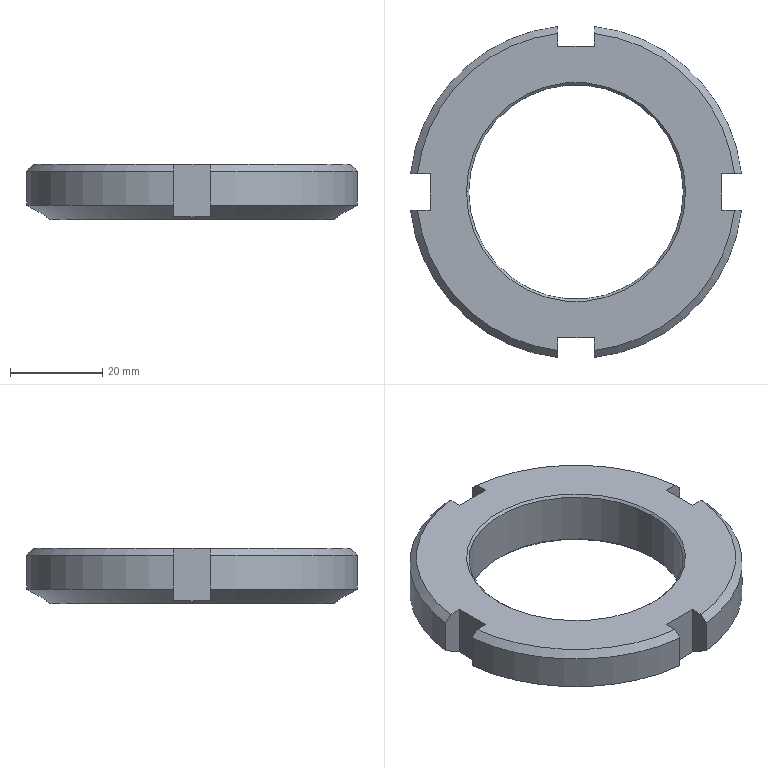Part | SolidWorks | features Chamfer 3, CirPattern 1, Cut 1, Extrusion 1 | 1 solid | 30 faces | box 71.554 x 71.554 x 12 mm | volume 25041 mm3 | plane 14 | cone 10 | cylinder 6 | commonest cylinder face diameters 72 x4 46.376 x2
STEP:
#1=CARTESIAN_POINT('',(-23.188,0.,11.5));
#2=VERTEX_POINT('',#1);
#3=CARTESIAN_POINT('',(23.188,0.,11.5));
#4=VERTEX_POINT('',#3);
#5=CARTESIAN_POINT('',(0.,0.,11.5));
#6=DIRECTION('',(0.,0.,1.));
#7=DIRECTION('',(1.,0.,0.));
#8=AXIS2_PLACEMENT_3D('',#5,#6,#7);
#9=CIRCLE('',#8,23.188);
#10=EDGE_CURVE('',#2,#4,#9,.T.);
#11=ORIENTED_EDGE('',*,*,#10,.F.);
#12=CARTESIAN_POINT('',(-23.688,0.,12.));
#13=VERTEX_POINT('',#12);
#14=CARTESIAN_POINT('',(-23.188,0.,11.5));
#15=DIRECTION('',(-0.7071,0.,0.7071));
#16=VECTOR('',#15,1000.);
#17=LINE('',#14,#16);
#18=EDGE_CURVE('',#2,#13,#17,.T.);
#19=ORIENTED_EDGE('',*,*,#18,.T.);
#20=CARTESIAN_POINT('',(23.688,0.,12.));
#21=VERTEX_POINT('',#20);
#22=CARTESIAN_POINT('',(0.,0.,12.));
#23=DIRECTION('',(0.,0.,-1.));
#24=DIRECTION('',(1.,0.,0.));
#25=AXIS2_PLACEMENT_3D('',#22,#23,#24);
#26=CIRCLE('',#25,23.688);
#27=EDGE_CURVE('',#21,#13,#26,.T.);
#28=ORIENTED_EDGE('',*,*,#27,.F.);
#29=CARTESIAN_POINT('',(23.188,0.,11.5));
#30=DIRECTION('',(0.7071,0.,0.7071));
#31=VECTOR('',#30,1000.);
#32=LINE('',#29,#31);
#33=EDGE_CURVE('',#4,#21,#32,.T.);
#34=ORIENTED_EDGE('',*,*,#33,.F.);
#35=EDGE_LOOP('',(#11,#19,#28,#34));
#36=FACE_OUTER_BOUND('',#35,.T.);
#37=CARTESIAN_POINT('',(0.,0.,11.5));
#38=DIRECTION('',(0.,0.,1.));
#39=DIRECTION('',(1.,0.,0.));
#40=AXIS2_PLACEMENT_3D('',#37,#38,#39);
#41=CONICAL_SURFACE('',#40,23.188,0.7854);
#42=ADVANCED_FACE('',(#36),#41,.F.);
#43=CARTESIAN_POINT('',(23.188,0.,0.5));
#44=VERTEX_POINT('',#43);
#45=CARTESIAN_POINT('',(-23.188,0.,0.5));
#46=VERTEX_POINT('',#45);
#47=CARTESIAN_POINT('',(0.,0.,0.5));
#48=DIRECTION('',(0.,0.,-1.));
#49=DIRECTION('',(1.,0.,0.));
#50=AXIS2_PLACEMENT_3D('',#47,#48,#49);
#51=CIRCLE('',#50,23.188);
#52=EDGE_CURVE('',#44,#46,#51,.T.);
#53=ORIENTED_EDGE('',*,*,#52,.F.);
#54=CARTESIAN_POINT('',(23.688,0.,0.));
#55=VERTEX_POINT('',#54);
#56=CARTESIAN_POINT('',(23.688,0.,0.));
#57=DIRECTION('',(0.7071,0.,-0.7071));
#58=VECTOR('',#57,1000.);
#59=LINE('',#56,#58);
#60=EDGE_CURVE('',#44,#55,#59,.T.);
#61=ORIENTED_EDGE('',*,*,#60,.T.);
#62=CARTESIAN_POINT('',(-23.688,0.,0.));
#63=VERTEX_POINT('',#62);
#64=CARTESIAN_POINT('',(0.,0.,0.));
#65=DIRECTION('',(0.,0.,1.));
#66=DIRECTION('',(1.,0.,0.));
#67=AXIS2_PLACEMENT_3D('',#64,#65,#66);
#68=CIRCLE('',#67,23.688);
#69=EDGE_CURVE('',#63,#55,#68,.T.);
#70=ORIENTED_EDGE('',*,*,#69,.F.);
#71=CARTESIAN_POINT('',(-23.688,0.,0.));
#72=DIRECTION('',(-0.7071,0.,-0.7071));
#73=VECTOR('',#72,1000.);
#74=LINE('',#71,#73);
#75=EDGE_CURVE('',#46,#63,#74,.T.);
#76=ORIENTED_EDGE('',*,*,#75,.F.);
#77=EDGE_LOOP('',(#53,#61,#70,#76));
#78=FACE_OUTER_BOUND('',#77,.T.);
#79=CARTESIAN_POINT('',(0.,0.,0.));
#80=DIRECTION('',(0.,0.,-1.));
#81=DIRECTION('',(-1.,0.,0.));
#82=AXIS2_PLACEMENT_3D('',#79,#80,#81);
#83=CONICAL_SURFACE('',#82,23.688,0.7854);
#84=ADVANCED_FACE('',(#78),#83,.F.);
#85=CARTESIAN_POINT('',(-30.5,0.,0.));
#86=VERTEX_POINT('',#85);
#87=CARTESIAN_POINT('',(30.5,0.,0.));
#88=VERTEX_POINT('',#87);
#89=CARTESIAN_POINT('',(0.,0.,0.));
#90=DIRECTION('',(0.,0.,-1.));
#91=DIRECTION('',(1.,0.,0.));
#92=AXIS2_PLACEMENT_3D('',#89,#90,#91);
#93=CIRCLE('',#92,30.5);
#94=EDGE_CURVE('',#86,#88,#93,.T.);
#95=ORIENTED_EDGE('',*,*,#94,.F.);
#96=CARTESIAN_POINT('',(-31.527,0.,0.593));
#97=VERTEX_POINT('',#96);
#98=CARTESIAN_POINT('',(-36.,0.,3.175));
#99=DIRECTION('',(-0.866,0.,0.5));
#100=VECTOR('',#99,1000.);
#101=LINE('',#98,#100);
#102=EDGE_CURVE('',#86,#97,#101,.T.);
#103=ORIENTED_EDGE('',*,*,#102,.T.);
#104=CARTESIAN_POINT('',(-31.527,4.,0.7389));
#105=VERTEX_POINT('',#104);
#106=CARTESIAN_POINT('',(-31.527,4.,0.7389));
#107=CARTESIAN_POINT('',(-31.527,2.671,0.6424));
#108=CARTESIAN_POINT('',(-31.527,1.338,0.593));
#109=CARTESIAN_POINT('',(-31.527,0.,0.593));
#110=B_SPLINE_CURVE_WITH_KNOTS('',3,(#106,#107,#108,#109),.UNSPECIFIED.,.F.,.F.,(4,4),(0.01045,0.01444),.UNSPECIFIED.);
#111=EDGE_CURVE('',#105,#97,#110,.T.);
#112=ORIENTED_EDGE('',*,*,#111,.F.);
#113=CARTESIAN_POINT('',(-35.777,4.,3.175));
#114=VERTEX_POINT('',#113);
#115=CARTESIAN_POINT('',(-35.777,4.,3.175));
#116=CARTESIAN_POINT('',(-34.361,4.,2.363));
#117=CARTESIAN_POINT('',(-32.944,4.,1.551));
#118=CARTESIAN_POINT('',(-31.527,4.,0.7389));
#119=B_SPLINE_CURVE_WITH_KNOTS('',3,(#115,#116,#117,#118),.UNSPECIFIED.,.F.,.F.,(4,4),(0.009232,0.01413),.UNSPECIFIED.);
#120=EDGE_CURVE('',#114,#105,#119,.T.);
#121=ORIENTED_EDGE('',*,*,#120,.F.);
#122=CARTESIAN_POINT('',(-4.,35.777,3.175));
#123=VERTEX_POINT('',#122);
#124=CARTESIAN_POINT('',(0.,0.,3.175));
#125=DIRECTION('',(0.,0.,1.));
#126=DIRECTION('',(1.,0.,0.));
#127=AXIS2_PLACEMENT_3D('',#124,#125,#126);
#128=CIRCLE('',#127,36.);
#129=EDGE_CURVE('',#123,#114,#128,.T.);
#130=ORIENTED_EDGE('',*,*,#129,.F.);
#131=CARTESIAN_POINT('',(-4.,31.527,0.7389));
#132=VERTEX_POINT('',#131);
#133=CARTESIAN_POINT('',(-4.,31.527,0.7389));
#134=CARTESIAN_POINT('',(-4.,32.944,1.551));
#135=CARTESIAN_POINT('',(-4.,34.361,2.363));
#136=CARTESIAN_POINT('',(-4.,35.777,3.175));
#137=B_SPLINE_CURVE_WITH_KNOTS('',3,(#133,#134,#135,#136),.UNSPECIFIED.,.F.,.F.,(4,4),(0.009599,0.0145),.UNSPECIFIED.);
#138=EDGE_CURVE('',#132,#123,#137,.T.);
#139=ORIENTED_EDGE('',*,*,#138,.F.);
#140=CARTESIAN_POINT('',(4.,31.527,0.7389));
#141=VERTEX_POINT('',#140);
#142=CARTESIAN_POINT('',(4.,31.527,0.7389));
#143=CARTESIAN_POINT('',(2.676,31.527,0.6427));
#144=CARTESIAN_POINT('',(1.347,31.527,0.5933));
#145=CARTESIAN_POINT('',(-0.6537,31.527,0.5928));
#146=CARTESIAN_POINT('',(-1.322,31.527,0.6049));
#147=CARTESIAN_POINT('',(-2.66,31.527,0.6536));
#148=CARTESIAN_POINT('',(-3.332,31.527,0.6903));
#149=CARTESIAN_POINT('',(-4.,31.527,0.7389));
#150=B_SPLINE_CURVE_WITH_KNOTS('',3,(#142,#143,#144,#145,#146,#147,#148,#149),.UNSPECIFIED.,.F.,.F.,(4,2,2,4),(0.01045,0.01443,0.01642,0.01841),.UNSPECIFIED.);
#151=EDGE_CURVE('',#141,#132,#150,.T.);
#152=ORIENTED_EDGE('',*,*,#151,.F.);
#153=CARTESIAN_POINT('',(4.,35.777,3.175));
#154=VERTEX_POINT('',#153);
#155=CARTESIAN_POINT('',(4.,35.777,3.175));
#156=CARTESIAN_POINT('',(4.,34.361,2.363));
#157=CARTESIAN_POINT('',(4.,32.944,1.551));
#158=CARTESIAN_POINT('',(4.,31.527,0.7389));
#159=B_SPLINE_CURVE_WITH_KNOTS('',3,(#155,#156,#157,#158),.UNSPECIFIED.,.F.,.F.,(4,4),(0.005677,0.01058),.UNSPECIFIED.);
#160=EDGE_CURVE('',#154,#141,#159,.T.);
#161=ORIENTED_EDGE('',*,*,#160,.F.);
#162=CARTESIAN_POINT('',(35.777,4.,3.175));
#163=VERTEX_POINT('',#162);
#164=CARTESIAN_POINT('',(0.,0.,3.175));
#165=DIRECTION('',(0.,0.,1.));
#166=DIRECTION('',(1.,0.,0.));
#167=AXIS2_PLACEMENT_3D('',#164,#165,#166);
#168=CIRCLE('',#167,36.);
#169=EDGE_CURVE('',#163,#154,#168,.T.);
#170=ORIENTED_EDGE('',*,*,#169,.F.);
#171=CARTESIAN_POINT('',(31.527,4.,0.7389));
#172=VERTEX_POINT('',#171);
#173=CARTESIAN_POINT('',(31.527,4.,0.7389));
#174=CARTESIAN_POINT('',(32.944,4.,1.551));
#175=CARTESIAN_POINT('',(34.361,4.,2.363));
#176=CARTESIAN_POINT('',(35.777,4.,3.175));
#177=B_SPLINE_CURVE_WITH_KNOTS('',3,(#173,#174,#175,#176),.UNSPECIFIED.,.F.,.F.,(4,4),(0.009599,0.0145),.UNSPECIFIED.);
#178=EDGE_CURVE('',#172,#163,#177,.T.);
#179=ORIENTED_EDGE('',*,*,#178,.F.);
#180=CARTESIAN_POINT('',(31.527,0.,0.593));
#181=VERTEX_POINT('',#180);
#182=CARTESIAN_POINT('',(31.527,0.,0.593));
#183=CARTESIAN_POINT('',(31.527,1.338,0.593));
#184=CARTESIAN_POINT('',(31.527,2.671,0.6424));
#185=CARTESIAN_POINT('',(31.527,4.,0.7389));
#186=B_SPLINE_CURVE_WITH_KNOTS('',3,(#182,#183,#184,#185),.UNSPECIFIED.,.F.,.F.,(4,4),(0.02046,0.02447),.UNSPECIFIED.);
#187=EDGE_CURVE('',#181,#172,#186,.T.);
#188=ORIENTED_EDGE('',*,*,#187,.F.);
#189=CARTESIAN_POINT('',(36.,0.,3.175));
#190=DIRECTION('',(0.866,0.,0.5));
#191=VECTOR('',#190,1000.);
#192=LINE('',#189,#191);
#193=EDGE_CURVE('',#88,#181,#192,.T.);
#194=ORIENTED_EDGE('',*,*,#193,.F.);
#195=EDGE_LOOP('',(#95,#103,#112,#121,#130,#139,#152,#161,#170,#179,#188,#194));
#196=FACE_OUTER_BOUND('',#195,.T.);
#197=CARTESIAN_POINT('',(0.,0.,3.175));
#198=DIRECTION('',(0.,0.,1.));
#199=DIRECTION('',(1.,0.,0.));
#200=AXIS2_PLACEMENT_3D('',#197,#198,#199);
#201=CONICAL_SURFACE('',#200,36.,1.047);
#202=ADVANCED_FACE('',(#196),#201,.T.);
#203=ORIENTED_EDGE('',*,*,#10,.T.);
#204=CARTESIAN_POINT('',(23.188,0.,12.));
#205=DIRECTION('',(0.,0.,-1.));
#206=VECTOR('',#205,1000.);
#207=LINE('',#204,#206);
#208=EDGE_CURVE('',#4,#44,#207,.T.);
#209=ORIENTED_EDGE('',*,*,#208,.T.);
#210=ORIENTED_EDGE('',*,*,#52,.T.);
#211=CARTESIAN_POINT('',(-23.188,0.,12.));
#212=DIRECTION('',(0.,0.,-1.));
#213=VECTOR('',#212,1000.);
#214=LINE('',#211,#213);
#215=EDGE_CURVE('',#2,#46,#214,.T.);
#216=ORIENTED_EDGE('',*,*,#215,.F.);
#217=EDGE_LOOP('',(#203,#209,#210,#216));
#218=FACE_OUTER_BOUND('',#217,.T.);
#219=CARTESIAN_POINT('',(0.,0.,12.));
#220=DIRECTION('',(0.,0.,-1.));
#221=DIRECTION('',(-1.,0.,0.));
#222=AXIS2_PLACEMENT_3D('',#219,#220,#221);
#223=CYLINDRICAL_SURFACE('',#222,23.188);
#224=ADVANCED_FACE('',(#218),#223,.F.);
#225=CARTESIAN_POINT('',(4.,35.777,10.5));
#226=VERTEX_POINT('',#225);
#227=CARTESIAN_POINT('',(35.777,4.,10.5));
#228=VERTEX_POINT('',#227);
#229=CARTESIAN_POINT('',(0.,0.,10.5));
#230=DIRECTION('',(0.,0.,-1.));
#231=DIRECTION('',(1.,0.,0.));
#232=AXIS2_PLACEMENT_3D('',#229,#230,#231);
#233=CIRCLE('',#232,36.);
#234=EDGE_CURVE('',#226,#228,#233,.T.);
#235=ORIENTED_EDGE('',*,*,#234,.T.);
#236=CARTESIAN_POINT('',(35.777,4.,0.));
#237=DIRECTION('',(0.,0.,1.));
#238=VECTOR('',#237,1000.);
#239=LINE('',#236,#238);
#240=EDGE_CURVE('',#163,#228,#239,.T.);
#241=ORIENTED_EDGE('',*,*,#240,.F.);
#242=ORIENTED_EDGE('',*,*,#169,.T.);
#243=CARTESIAN_POINT('',(4.,35.777,0.));
#244=DIRECTION('',(0.,0.,1.));
#245=VECTOR('',#244,1000.);
#246=LINE('',#243,#245);
#247=EDGE_CURVE('',#154,#226,#246,.T.);
#248=ORIENTED_EDGE('',*,*,#247,.T.);
#249=EDGE_LOOP('',(#235,#241,#242,#248));
#250=FACE_OUTER_BOUND('',#249,.T.);
#251=CARTESIAN_POINT('',(0.,0.,12.));
#252=DIRECTION('',(0.,0.,-1.));
#253=DIRECTION('',(-1.,0.,0.));
#254=AXIS2_PLACEMENT_3D('',#251,#252,#253);
#255=CYLINDRICAL_SURFACE('',#254,36.);
#256=ADVANCED_FACE('',(#250),#255,.T.);
#257=CARTESIAN_POINT('',(34.267,4.,12.));
#258=VERTEX_POINT('',#257);
#259=CARTESIAN_POINT('',(35.777,4.,10.5));
#260=CARTESIAN_POINT('',(35.385,4.,10.89));
#261=CARTESIAN_POINT('',(34.992,4.,11.28));
#262=CARTESIAN_POINT('',(34.6,4.,11.67));
#263=CARTESIAN_POINT('',(34.489,4.,11.78));
#264=CARTESIAN_POINT('',(34.378,4.,11.89));
#265=CARTESIAN_POINT('',(34.267,4.,12.));
#266=B_SPLINE_CURVE_WITH_KNOTS('',3,(#259,#260,#261,#262,#263,#264,#265),.UNSPECIFIED.,.F.,.F.,(4,3,4),(0.007216,0.008875,0.009344),.UNSPECIFIED.);
#267=EDGE_CURVE('',#228,#258,#266,.T.);
#268=ORIENTED_EDGE('',*,*,#267,.F.);
#269=ORIENTED_EDGE('',*,*,#234,.F.);
#270=CARTESIAN_POINT('',(4.,34.267,12.));
#271=VERTEX_POINT('',#270);
#272=CARTESIAN_POINT('',(4.,34.267,12.));
#273=CARTESIAN_POINT('',(4.,34.378,11.89));
#274=CARTESIAN_POINT('',(4.,34.489,11.78));
#275=CARTESIAN_POINT('',(4.,34.6,11.67));
#276=CARTESIAN_POINT('',(4.,34.992,11.28));
#277=CARTESIAN_POINT('',(4.,35.385,10.89));
#278=CARTESIAN_POINT('',(4.,35.777,10.5));
#279=B_SPLINE_CURVE_WITH_KNOTS('',3,(#272,#273,#274,#275,#276,#277,#278),.UNSPECIFIED.,.F.,.F.,(4,3,4),(0.008406,0.008875,0.01053),.UNSPECIFIED.);
#280=EDGE_CURVE('',#271,#226,#279,.T.);
#281=ORIENTED_EDGE('',*,*,#280,.F.);
#282=CARTESIAN_POINT('',(0.,0.,12.));
#283=DIRECTION('',(0.,0.,1.));
#284=DIRECTION('',(1.,0.,0.));
#285=AXIS2_PLACEMENT_3D('',#282,#283,#284);
#286=CIRCLE('',#285,34.5);
#287=EDGE_CURVE('',#258,#271,#286,.T.);
#288=ORIENTED_EDGE('',*,*,#287,.F.);
#289=EDGE_LOOP('',(#268,#269,#281,#288));
#290=FACE_OUTER_BOUND('',#289,.T.);
#291=CARTESIAN_POINT('',(0.,0.,12.));
#292=DIRECTION('',(0.,0.,-1.));
#293=DIRECTION('',(-1.,0.,0.));
#294=AXIS2_PLACEMENT_3D('',#291,#292,#293);
#295=CONICAL_SURFACE('',#294,34.5,0.7854);
#296=ADVANCED_FACE('',(#290),#295,.T.);
#297=CARTESIAN_POINT('',(-35.777,4.,10.5));
#298=VERTEX_POINT('',#297);
#299=CARTESIAN_POINT('',(-4.,35.777,10.5));
#300=VERTEX_POINT('',#299);
#301=CARTESIAN_POINT('',(0.,0.,10.5));
#302=DIRECTION('',(0.,0.,-1.));
#303=DIRECTION('',(1.,0.,0.));
#304=AXIS2_PLACEMENT_3D('',#301,#302,#303);
#305=CIRCLE('',#304,36.);
#306=EDGE_CURVE('',#298,#300,#305,.T.);
#307=ORIENTED_EDGE('',*,*,#306,.T.);
#308=CARTESIAN_POINT('',(-4.,35.777,0.));
#309=DIRECTION('',(0.,0.,1.));
#310=VECTOR('',#309,1000.);
#311=LINE('',#308,#310);
#312=EDGE_CURVE('',#123,#300,#311,.T.);
#313=ORIENTED_EDGE('',*,*,#312,.F.);
#314=ORIENTED_EDGE('',*,*,#129,.T.);
#315=CARTESIAN_POINT('',(-35.777,4.,0.));
#316=DIRECTION('',(0.,0.,1.));
#317=VECTOR('',#316,1000.);
#318=LINE('',#315,#317);
#319=EDGE_CURVE('',#114,#298,#318,.T.);
#320=ORIENTED_EDGE('',*,*,#319,.T.);
#321=EDGE_LOOP('',(#307,#313,#314,#320));
#322=FACE_OUTER_BOUND('',#321,.T.);
#323=CARTESIAN_POINT('',(0.,0.,12.));
#324=DIRECTION('',(0.,0.,-1.));
#325=DIRECTION('',(-1.,0.,0.));
#326=AXIS2_PLACEMENT_3D('',#323,#324,#325);
#327=CYLINDRICAL_SURFACE('',#326,36.);
#328=ADVANCED_FACE('',(#322),#327,.T.);
#329=CARTESIAN_POINT('',(-4.,34.267,12.));
#330=VERTEX_POINT('',#329);
#331=CARTESIAN_POINT('',(-4.,35.777,10.5));
#332=CARTESIAN_POINT('',(-4.,35.385,10.89));
#333=CARTESIAN_POINT('',(-4.,34.992,11.28));
#334=CARTESIAN_POINT('',(-4.,34.6,11.67));
#335=CARTESIAN_POINT('',(-4.,34.489,11.78));
#336=CARTESIAN_POINT('',(-4.,34.378,11.89));
#337=CARTESIAN_POINT('',(-4.,34.267,12.));
#338=B_SPLINE_CURVE_WITH_KNOTS('',3,(#331,#332,#333,#334,#335,#336,#337),.UNSPECIFIED.,.F.,.F.,(4,3,4),(0.007216,0.008875,0.009344),.UNSPECIFIED.);
#339=EDGE_CURVE('',#300,#330,#338,.T.);
#340=ORIENTED_EDGE('',*,*,#339,.F.);
#341=ORIENTED_EDGE('',*,*,#306,.F.);
#342=CARTESIAN_POINT('',(-34.267,4.,12.));
#343=VERTEX_POINT('',#342);
#344=CARTESIAN_POINT('',(-34.267,4.,12.));
#345=CARTESIAN_POINT('',(-34.557,4.,11.713));
#346=CARTESIAN_POINT('',(-34.846,4.,11.426));
#347=CARTESIAN_POINT('',(-35.135,4.,11.138));
#348=CARTESIAN_POINT('',(-35.349,4.,10.926));
#349=CARTESIAN_POINT('',(-35.563,4.,10.713));
#350=CARTESIAN_POINT('',(-35.777,4.,10.5));
#351=B_SPLINE_CURVE_WITH_KNOTS('',3,(#344,#345,#346,#347,#348,#349,#350),.UNSPECIFIED.,.F.,.F.,(4,3,4),(0.007653,0.008875,0.009781),.UNSPECIFIED.);
#352=EDGE_CURVE('',#343,#298,#351,.T.);
#353=ORIENTED_EDGE('',*,*,#352,.F.);
#354=CARTESIAN_POINT('',(0.,0.,12.));
#355=DIRECTION('',(0.,0.,1.));
#356=DIRECTION('',(1.,0.,0.));
#357=AXIS2_PLACEMENT_3D('',#354,#355,#356);
#358=CIRCLE('',#357,34.5);
#359=EDGE_CURVE('',#330,#343,#358,.T.);
#360=ORIENTED_EDGE('',*,*,#359,.F.);
#361=EDGE_LOOP('',(#340,#341,#353,#360));
#362=FACE_OUTER_BOUND('',#361,.T.);
#363=CARTESIAN_POINT('',(0.,0.,12.));
#364=DIRECTION('',(0.,0.,-1.));
#365=DIRECTION('',(-1.,0.,0.));
#366=AXIS2_PLACEMENT_3D('',#363,#364,#365);
#367=CONICAL_SURFACE('',#366,34.5,0.7854);
#368=ADVANCED_FACE('',(#362),#367,.T.);
#369=CARTESIAN_POINT('',(-4.,-35.777,10.5));
#370=VERTEX_POINT('',#369);
#371=CARTESIAN_POINT('',(-35.777,-4.,10.5));
#372=VERTEX_POINT('',#371);
#373=CARTESIAN_POINT('',(0.,0.,10.5));
#374=DIRECTION('',(0.,0.,-1.));
#375=DIRECTION('',(1.,0.,0.));
#376=AXIS2_PLACEMENT_3D('',#373,#374,#375);
#377=CIRCLE('',#376,36.);
#378=EDGE_CURVE('',#370,#372,#377,.T.);
#379=ORIENTED_EDGE('',*,*,#378,.T.);
#380=CARTESIAN_POINT('',(-35.777,-4.,3.175));
#381=VERTEX_POINT('',#380);
#382=CARTESIAN_POINT('',(-35.777,-4.,0.));
#383=DIRECTION('',(0.,0.,1.));
#384=VECTOR('',#383,1000.);
#385=LINE('',#382,#384);
#386=EDGE_CURVE('',#381,#372,#385,.T.);
#387=ORIENTED_EDGE('',*,*,#386,.F.);
#388=CARTESIAN_POINT('',(-4.,-35.777,3.175));
#389=VERTEX_POINT('',#388);
#390=CARTESIAN_POINT('',(0.,0.,3.175));
#391=DIRECTION('',(0.,0.,1.));
#392=DIRECTION('',(1.,0.,0.));
#393=AXIS2_PLACEMENT_3D('',#390,#391,#392);
#394=CIRCLE('',#393,36.);
#395=EDGE_CURVE('',#381,#389,#394,.T.);
#396=ORIENTED_EDGE('',*,*,#395,.T.);
#397=CARTESIAN_POINT('',(-4.,-35.777,0.));
#398=DIRECTION('',(0.,0.,1.));
#399=VECTOR('',#398,1000.);
#400=LINE('',#397,#399);
#401=EDGE_CURVE('',#389,#370,#400,.T.);
#402=ORIENTED_EDGE('',*,*,#401,.T.);
#403=EDGE_LOOP('',(#379,#387,#396,#402));
#404=FACE_OUTER_BOUND('',#403,.T.);
#405=CARTESIAN_POINT('',(0.,0.,12.));
#406=DIRECTION('',(0.,0.,-1.));
#407=DIRECTION('',(-1.,0.,0.));
#408=AXIS2_PLACEMENT_3D('',#405,#406,#407);
#409=CYLINDRICAL_SURFACE('',#408,36.);
#410=ADVANCED_FACE('',(#404),#409,.T.);
#411=CARTESIAN_POINT('',(-34.267,-4.,12.));
#412=VERTEX_POINT('',#411);
#413=CARTESIAN_POINT('',(-35.777,-4.,10.5));
#414=CARTESIAN_POINT('',(-35.563,-4.,10.713));
#415=CARTESIAN_POINT('',(-35.349,-4.,10.926));
#416=CARTESIAN_POINT('',(-35.135,-4.,11.138));
#417=CARTESIAN_POINT('',(-34.846,-4.,11.426));
#418=CARTESIAN_POINT('',(-34.557,-4.,11.713));
#419=CARTESIAN_POINT('',(-34.267,-4.,12.));
#420=B_SPLINE_CURVE_WITH_KNOTS('',3,(#413,#414,#415,#416,#417,#418,#419),.UNSPECIFIED.,.F.,.F.,(4,3,4),(0.00797,0.008875,0.0101),.UNSPECIFIED.);
#421=EDGE_CURVE('',#372,#412,#420,.T.);
#422=ORIENTED_EDGE('',*,*,#421,.F.);
#423=ORIENTED_EDGE('',*,*,#378,.F.);
#424=CARTESIAN_POINT('',(-4.,-34.267,12.));
#425=VERTEX_POINT('',#424);
#426=CARTESIAN_POINT('',(-4.,-34.267,12.));
#427=CARTESIAN_POINT('',(-4.,-34.557,11.713));
#428=CARTESIAN_POINT('',(-4.,-34.846,11.426));
#429=CARTESIAN_POINT('',(-4.,-35.135,11.138));
#430=CARTESIAN_POINT('',(-4.,-35.349,10.926));
#431=CARTESIAN_POINT('',(-4.,-35.563,10.713));
#432=CARTESIAN_POINT('',(-4.,-35.777,10.5));
#433=B_SPLINE_CURVE_WITH_KNOTS('',3,(#426,#427,#428,#429,#430,#431,#432),.UNSPECIFIED.,.F.,.F.,(4,3,4),(0.007653,0.008875,0.009781),.UNSPECIFIED.);
#434=EDGE_CURVE('',#425,#370,#433,.T.);
#435=ORIENTED_EDGE('',*,*,#434,.F.);
#436=CARTESIAN_POINT('',(0.,0.,12.));
#437=DIRECTION('',(0.,0.,1.));
#438=DIRECTION('',(1.,0.,0.));
#439=AXIS2_PLACEMENT_3D('',#436,#437,#438);
#440=CIRCLE('',#439,34.5);
#441=EDGE_CURVE('',#412,#425,#440,.T.);
#442=ORIENTED_EDGE('',*,*,#441,.F.);
#443=EDGE_LOOP('',(#422,#423,#435,#442));
#444=FACE_OUTER_BOUND('',#443,.T.);
#445=CARTESIAN_POINT('',(0.,0.,12.));
#446=DIRECTION('',(0.,0.,-1.));
#447=DIRECTION('',(-1.,0.,0.));
#448=AXIS2_PLACEMENT_3D('',#445,#446,#447);
#449=CONICAL_SURFACE('',#448,34.5,0.7854);
#450=ADVANCED_FACE('',(#444),#449,.T.);
#451=ORIENTED_EDGE('',*,*,#27,.T.);
#452=CARTESIAN_POINT('',(0.,0.,12.));
#453=DIRECTION('',(0.,0.,-1.));
#454=DIRECTION('',(1.,0.,0.));
#455=AXIS2_PLACEMENT_3D('',#452,#453,#454);
#456=CIRCLE('',#455,23.688);
#457=EDGE_CURVE('',#13,#21,#456,.T.);
#458=ORIENTED_EDGE('',*,*,#457,.T.);
#459=EDGE_LOOP('',(#451,#458));
#460=FACE_BOUND('',#459,.T.);
#461=CARTESIAN_POINT('',(31.527,4.,12.));
#462=VERTEX_POINT('',#461);
#463=CARTESIAN_POINT('',(31.527,4.,12.));
#464=DIRECTION('',(-1.,0.,0.));
#465=VECTOR('',#464,1000.);
#466=LINE('',#463,#465);
#467=EDGE_CURVE('',#258,#462,#466,.T.);
#468=ORIENTED_EDGE('',*,*,#467,.F.);
#469=ORIENTED_EDGE('',*,*,#287,.T.);
#470=CARTESIAN_POINT('',(4.,31.527,12.));
#471=VERTEX_POINT('',#470);
#472=CARTESIAN_POINT('',(4.,31.527,12.));
#473=DIRECTION('',(0.,1.,0.));
#474=VECTOR('',#473,1000.);
#475=LINE('',#472,#474);
#476=EDGE_CURVE('',#471,#271,#475,.T.);
#477=ORIENTED_EDGE('',*,*,#476,.F.);
#478=CARTESIAN_POINT('',(-4.,31.527,12.));
#479=VERTEX_POINT('',#478);
#480=CARTESIAN_POINT('',(4.,31.527,12.));
#481=DIRECTION('',(1.,0.,0.));
#482=VECTOR('',#481,1000.);
#483=LINE('',#480,#482);
#484=EDGE_CURVE('',#479,#471,#483,.T.);
#485=ORIENTED_EDGE('',*,*,#484,.F.);
#486=CARTESIAN_POINT('',(-4.,31.527,12.));
#487=DIRECTION('',(0.,-1.,0.));
#488=VECTOR('',#487,1000.);
#489=LINE('',#486,#488);
#490=EDGE_CURVE('',#330,#479,#489,.T.);
#491=ORIENTED_EDGE('',*,*,#490,.F.);
#492=ORIENTED_EDGE('',*,*,#359,.T.);
#493=CARTESIAN_POINT('',(-31.527,4.,12.));
#494=VERTEX_POINT('',#493);
#495=CARTESIAN_POINT('',(-31.527,4.,12.));
#496=DIRECTION('',(-1.,0.,0.));
#497=VECTOR('',#496,1000.);
#498=LINE('',#495,#497);
#499=EDGE_CURVE('',#494,#343,#498,.T.);
#500=ORIENTED_EDGE('',*,*,#499,.F.);
#501=CARTESIAN_POINT('',(-31.527,-4.,12.));
#502=VERTEX_POINT('',#501);
#503=CARTESIAN_POINT('',(-31.527,4.,12.));
#504=DIRECTION('',(0.,1.,0.));
#505=VECTOR('',#504,1000.);
#506=LINE('',#503,#505);
#507=EDGE_CURVE('',#502,#494,#506,.T.);
#508=ORIENTED_EDGE('',*,*,#507,.F.);
#509=CARTESIAN_POINT('',(-31.527,-4.,12.));
#510=DIRECTION('',(1.,0.,0.));
#511=VECTOR('',#510,1000.);
#512=LINE('',#509,#511);
#513=EDGE_CURVE('',#412,#502,#512,.T.);
#514=ORIENTED_EDGE('',*,*,#513,.F.);
#515=ORIENTED_EDGE('',*,*,#441,.T.);
#516=CARTESIAN_POINT('',(-4.,-31.527,12.));
#517=VERTEX_POINT('',#516);
#518=CARTESIAN_POINT('',(-4.,-31.527,12.));
#519=DIRECTION('',(0.,-1.,0.));
#520=VECTOR('',#519,1000.);
#521=LINE('',#518,#520);
#522=EDGE_CURVE('',#517,#425,#521,.T.);
#523=ORIENTED_EDGE('',*,*,#522,.F.);
#524=CARTESIAN_POINT('',(4.,-31.527,12.));
#525=VERTEX_POINT('',#524);
#526=CARTESIAN_POINT('',(-4.,-31.527,12.));
#527=DIRECTION('',(-1.,0.,0.));
#528=VECTOR('',#527,1000.);
#529=LINE('',#526,#528);
#530=EDGE_CURVE('',#525,#517,#529,.T.);
#531=ORIENTED_EDGE('',*,*,#530,.F.);
#532=CARTESIAN_POINT('',(4.,-34.267,12.));
#533=VERTEX_POINT('',#532);
#534=CARTESIAN_POINT('',(4.,-31.527,12.));
#535=DIRECTION('',(0.,1.,0.));
#536=VECTOR('',#535,1000.);
#537=LINE('',#534,#536);
#538=EDGE_CURVE('',#533,#525,#537,.T.);
#539=ORIENTED_EDGE('',*,*,#538,.F.);
#540=CARTESIAN_POINT('',(34.267,-4.,12.));
#541=VERTEX_POINT('',#540);
#542=CARTESIAN_POINT('',(0.,0.,12.));
#543=DIRECTION('',(0.,0.,1.));
#544=DIRECTION('',(1.,0.,0.));
#545=AXIS2_PLACEMENT_3D('',#542,#543,#544);
#546=CIRCLE('',#545,34.5);
#547=EDGE_CURVE('',#533,#541,#546,.T.);
#548=ORIENTED_EDGE('',*,*,#547,.T.);
#549=CARTESIAN_POINT('',(31.527,-4.,12.));
#550=VERTEX_POINT('',#549);
#551=CARTESIAN_POINT('',(31.527,-4.,12.));
#552=DIRECTION('',(1.,0.,0.));
#553=VECTOR('',#552,1000.);
#554=LINE('',#551,#553);
#555=EDGE_CURVE('',#550,#541,#554,.T.);
#556=ORIENTED_EDGE('',*,*,#555,.F.);
#557=CARTESIAN_POINT('',(31.527,-4.,12.));
#558=DIRECTION('',(0.,-1.,0.));
#559=VECTOR('',#558,1000.);
#560=LINE('',#557,#559);
#561=EDGE_CURVE('',#462,#550,#560,.T.);
#562=ORIENTED_EDGE('',*,*,#561,.F.);
#563=EDGE_LOOP('',(#468,#469,#477,#485,#491,#492,#500,#508,#514,#515,#523,#531,#539,#548,#556,#562));
#564=FACE_OUTER_BOUND('',#563,.T.);
#565=CARTESIAN_POINT('',(0.,0.,12.));
#566=DIRECTION('',(0.,0.,1.));
#567=DIRECTION('',(1.,0.,0.));
#568=AXIS2_PLACEMENT_3D('',#565,#566,#567);
#569=PLANE('',#568);
#570=ADVANCED_FACE('',(#460,#564),#569,.T.);
#571=ORIENTED_EDGE('',*,*,#69,.T.);
#572=CARTESIAN_POINT('',(0.,0.,0.));
#573=DIRECTION('',(0.,0.,1.));
#574=DIRECTION('',(1.,0.,0.));
#575=AXIS2_PLACEMENT_3D('',#572,#573,#574);
#576=CIRCLE('',#575,23.688);
#577=EDGE_CURVE('',#55,#63,#576,.T.);
#578=ORIENTED_EDGE('',*,*,#577,.T.);
#579=EDGE_LOOP('',(#571,#578));
#580=FACE_BOUND('',#579,.T.);
#581=CARTESIAN_POINT('',(0.,0.,0.));
#582=DIRECTION('',(0.,0.,-1.));
#583=DIRECTION('',(1.,0.,0.));
#584=AXIS2_PLACEMENT_3D('',#581,#582,#583);
#585=CIRCLE('',#584,30.5);
#586=EDGE_CURVE('',#88,#86,#585,.T.);
#587=ORIENTED_EDGE('',*,*,#586,.T.);
#588=ORIENTED_EDGE('',*,*,#94,.T.);
#589=EDGE_LOOP('',(#587,#588));
#590=FACE_OUTER_BOUND('',#589,.T.);
#591=CARTESIAN_POINT('',(0.,0.,0.));
#592=DIRECTION('',(0.,0.,1.));
#593=DIRECTION('',(1.,0.,0.));
#594=AXIS2_PLACEMENT_3D('',#591,#592,#593);
#595=PLANE('',#594);
#596=ADVANCED_FACE('',(#580,#590),#595,.F.);
#597=CARTESIAN_POINT('',(4.,-35.777,3.175));
#598=VERTEX_POINT('',#597);
#599=CARTESIAN_POINT('',(35.777,-4.,3.175));
#600=VERTEX_POINT('',#599);
#601=CARTESIAN_POINT('',(0.,0.,3.175));
#602=DIRECTION('',(0.,0.,1.));
#603=DIRECTION('',(1.,0.,0.));
#604=AXIS2_PLACEMENT_3D('',#601,#602,#603);
#605=CIRCLE('',#604,36.);
#606=EDGE_CURVE('',#598,#600,#605,.T.);
#607=ORIENTED_EDGE('',*,*,#606,.T.);
#608=CARTESIAN_POINT('',(35.777,-4.,10.5));
#609=VERTEX_POINT('',#608);
#610=CARTESIAN_POINT('',(35.777,-4.,0.));
#611=DIRECTION('',(0.,0.,1.));
#612=VECTOR('',#611,1000.);
#613=LINE('',#610,#612);
#614=EDGE_CURVE('',#600,#609,#613,.T.);
#615=ORIENTED_EDGE('',*,*,#614,.T.);
#616=CARTESIAN_POINT('',(4.,-35.777,10.5));
#617=VERTEX_POINT('',#616);
#618=CARTESIAN_POINT('',(0.,0.,10.5));
#619=DIRECTION('',(0.,0.,-1.));
#620=DIRECTION('',(1.,0.,0.));
#621=AXIS2_PLACEMENT_3D('',#618,#619,#620);
#622=CIRCLE('',#621,36.);
#623=EDGE_CURVE('',#609,#617,#622,.T.);
#624=ORIENTED_EDGE('',*,*,#623,.T.);
#625=CARTESIAN_POINT('',(4.,-35.777,0.));
#626=DIRECTION('',(0.,0.,1.));
#627=VECTOR('',#626,1000.);
#628=LINE('',#625,#627);
#629=EDGE_CURVE('',#598,#617,#628,.T.);
#630=ORIENTED_EDGE('',*,*,#629,.F.);
#631=EDGE_LOOP('',(#607,#615,#624,#630));
#632=FACE_OUTER_BOUND('',#631,.T.);
#633=CARTESIAN_POINT('',(0.,0.,12.));
#634=DIRECTION('',(0.,0.,-1.));
#635=DIRECTION('',(-1.,0.,0.));
#636=AXIS2_PLACEMENT_3D('',#633,#634,#635);
#637=CYLINDRICAL_SURFACE('',#636,36.);
#638=ADVANCED_FACE('',(#632),#637,.T.);
#639=ORIENTED_EDGE('',*,*,#208,.F.);
#640=CARTESIAN_POINT('',(0.,0.,11.5));
#641=DIRECTION('',(0.,0.,1.));
#642=DIRECTION('',(1.,0.,0.));
#643=AXIS2_PLACEMENT_3D('',#640,#641,#642);
#644=CIRCLE('',#643,23.188);
#645=EDGE_CURVE('',#4,#2,#644,.T.);
#646=ORIENTED_EDGE('',*,*,#645,.T.);
#647=ORIENTED_EDGE('',*,*,#215,.T.);
#648=CARTESIAN_POINT('',(0.,0.,0.5));
#649=DIRECTION('',(0.,0.,-1.));
#650=DIRECTION('',(1.,0.,0.));
#651=AXIS2_PLACEMENT_3D('',#648,#649,#650);
#652=CIRCLE('',#651,23.188);
#653=EDGE_CURVE('',#46,#44,#652,.T.);
#654=ORIENTED_EDGE('',*,*,#653,.T.);
#655=EDGE_LOOP('',(#639,#646,#647,#654));
#656=FACE_OUTER_BOUND('',#655,.T.);
#657=CARTESIAN_POINT('',(0.,0.,12.));
#658=DIRECTION('',(0.,0.,-1.));
#659=DIRECTION('',(-1.,0.,0.));
#660=AXIS2_PLACEMENT_3D('',#657,#658,#659);
#661=CYLINDRICAL_SURFACE('',#660,23.188);
#662=ADVANCED_FACE('',(#656),#661,.F.);
#663=CARTESIAN_POINT('',(34.267,-4.,12.));
#664=CARTESIAN_POINT('',(34.378,-4.,11.89));
#665=CARTESIAN_POINT('',(34.489,-4.,11.78));
#666=CARTESIAN_POINT('',(34.6,-4.,11.67));
#667=CARTESIAN_POINT('',(34.992,-4.,11.28));
#668=CARTESIAN_POINT('',(35.385,-4.,10.89));
#669=CARTESIAN_POINT('',(35.777,-4.,10.5));
#670=B_SPLINE_CURVE_WITH_KNOTS('',3,(#663,#664,#665,#666,#667,#668,#669),.UNSPECIFIED.,.F.,.F.,(4,3,4),(0.008406,0.008875,0.01053),.UNSPECIFIED.);
#671=EDGE_CURVE('',#541,#609,#670,.T.);
#672=ORIENTED_EDGE('',*,*,#671,.F.);
#673=ORIENTED_EDGE('',*,*,#547,.F.);
#674=CARTESIAN_POINT('',(4.,-35.777,10.5));
#675=CARTESIAN_POINT('',(4.,-35.563,10.713));
#676=CARTESIAN_POINT('',(4.,-35.349,10.926));
#677=CARTESIAN_POINT('',(4.,-35.135,11.138));
#678=CARTESIAN_POINT('',(4.,-34.846,11.426));
#679=CARTESIAN_POINT('',(4.,-34.557,11.713));
#680=CARTESIAN_POINT('',(4.,-34.267,12.));
#681=B_SPLINE_CURVE_WITH_KNOTS('',3,(#674,#675,#676,#677,#678,#679,#680),.UNSPECIFIED.,.F.,.F.,(4,3,4),(0.00797,0.008875,0.0101),.UNSPECIFIED.);
#682=EDGE_CURVE('',#617,#533,#681,.T.);
#683=ORIENTED_EDGE('',*,*,#682,.F.);
#684=ORIENTED_EDGE('',*,*,#623,.F.);
#685=EDGE_LOOP('',(#672,#673,#683,#684));
#686=FACE_OUTER_BOUND('',#685,.T.);
#687=CARTESIAN_POINT('',(0.,0.,12.));
#688=DIRECTION('',(0.,0.,-1.));
#689=DIRECTION('',(-1.,0.,0.));
#690=AXIS2_PLACEMENT_3D('',#687,#688,#689);
#691=CONICAL_SURFACE('',#690,34.5,0.7854);
#692=ADVANCED_FACE('',(#686),#691,.T.);
#693=ORIENTED_EDGE('',*,*,#102,.F.);
#694=ORIENTED_EDGE('',*,*,#586,.F.);
#695=ORIENTED_EDGE('',*,*,#193,.T.);
#696=CARTESIAN_POINT('',(31.527,-4.,0.7389));
#697=VERTEX_POINT('',#696);
#698=CARTESIAN_POINT('',(31.527,-4.,0.7389));
#699=CARTESIAN_POINT('',(31.527,-3.334,0.6905));
#700=CARTESIAN_POINT('',(31.527,-2.665,0.6538));
#701=CARTESIAN_POINT('',(31.527,-1.331,0.6051));
#702=CARTESIAN_POINT('',(31.527,-0.6647,0.593));
#703=CARTESIAN_POINT('',(31.527,0.,0.593));
#704=B_SPLINE_CURVE_WITH_KNOTS('',3,(#698,#699,#700,#701,#702,#703),.UNSPECIFIED.,.F.,.F.,(4,2,4),(0.01648,0.01847,0.02046),.UNSPECIFIED.);
#705=EDGE_CURVE('',#697,#181,#704,.T.);
#706=ORIENTED_EDGE('',*,*,#705,.F.);
#707=CARTESIAN_POINT('',(35.777,-4.,3.175));
#708=CARTESIAN_POINT('',(34.361,-4.,2.363));
#709=CARTESIAN_POINT('',(32.944,-4.,1.551));
#710=CARTESIAN_POINT('',(31.527,-4.,0.7389));
#711=B_SPLINE_CURVE_WITH_KNOTS('',3,(#707,#708,#709,#710),.UNSPECIFIED.,.F.,.F.,(4,4),(0.005677,0.01058),.UNSPECIFIED.);
#712=EDGE_CURVE('',#600,#697,#711,.T.);
#713=ORIENTED_EDGE('',*,*,#712,.F.);
#714=ORIENTED_EDGE('',*,*,#606,.F.);
#715=CARTESIAN_POINT('',(4.,-31.527,0.7389));
#716=VERTEX_POINT('',#715);
#717=CARTESIAN_POINT('',(4.,-31.527,0.7389));
#718=CARTESIAN_POINT('',(4.,-32.944,1.551));
#719=CARTESIAN_POINT('',(4.,-34.361,2.363));
#720=CARTESIAN_POINT('',(4.,-35.777,3.175));
#721=B_SPLINE_CURVE_WITH_KNOTS('',3,(#717,#718,#719,#720),.UNSPECIFIED.,.F.,.F.,(4,4),(0.006045,0.01094),.UNSPECIFIED.);
#722=EDGE_CURVE('',#716,#598,#721,.T.);
#723=ORIENTED_EDGE('',*,*,#722,.F.);
#724=CARTESIAN_POINT('',(-4.,-31.527,0.7389));
#725=VERTEX_POINT('',#724);
#726=CARTESIAN_POINT('',(-4.,-31.527,0.7389));
#727=CARTESIAN_POINT('',(-3.332,-31.527,0.6903));
#728=CARTESIAN_POINT('',(-2.66,-31.527,0.6536));
#729=CARTESIAN_POINT('',(-1.322,-31.527,0.6049));
#730=CARTESIAN_POINT('',(-0.6537,-31.527,0.5928));
#731=CARTESIAN_POINT('',(1.347,-31.527,0.5933));
#732=CARTESIAN_POINT('',(2.676,-31.527,0.6427));
#733=CARTESIAN_POINT('',(4.,-31.527,0.7389));
#734=B_SPLINE_CURVE_WITH_KNOTS('',3,(#726,#727,#728,#729,#730,#731,#732,#733),.UNSPECIFIED.,.F.,.F.,(4,2,2,4),(0.01648,0.01848,0.02047,0.02447),.UNSPECIFIED.);
#735=EDGE_CURVE('',#725,#716,#734,.T.);
#736=ORIENTED_EDGE('',*,*,#735,.F.);
#737=CARTESIAN_POINT('',(-4.,-35.777,3.175));
#738=CARTESIAN_POINT('',(-4.,-34.361,2.363));
#739=CARTESIAN_POINT('',(-4.,-32.944,1.551));
#740=CARTESIAN_POINT('',(-4.,-31.527,0.7389));
#741=B_SPLINE_CURVE_WITH_KNOTS('',3,(#737,#738,#739,#740),.UNSPECIFIED.,.F.,.F.,(4,4),(0.009232,0.01413),.UNSPECIFIED.);
#742=EDGE_CURVE('',#389,#725,#741,.T.);
#743=ORIENTED_EDGE('',*,*,#742,.F.);
#744=ORIENTED_EDGE('',*,*,#395,.F.);
#745=CARTESIAN_POINT('',(-31.527,-4.,0.7389));
#746=VERTEX_POINT('',#745);
#747=CARTESIAN_POINT('',(-31.527,-4.,0.7389));
#748=CARTESIAN_POINT('',(-32.944,-4.,1.551));
#749=CARTESIAN_POINT('',(-34.361,-4.,2.363));
#750=CARTESIAN_POINT('',(-35.777,-4.,3.175));
#751=B_SPLINE_CURVE_WITH_KNOTS('',3,(#747,#748,#749,#750),.UNSPECIFIED.,.F.,.F.,(4,4),(0.006045,0.01094),.UNSPECIFIED.);
#752=EDGE_CURVE('',#746,#381,#751,.T.);
#753=ORIENTED_EDGE('',*,*,#752,.F.);
#754=CARTESIAN_POINT('',(-31.527,0.,0.593));
#755=CARTESIAN_POINT('',(-31.527,-0.6647,0.593));
#756=CARTESIAN_POINT('',(-31.527,-1.331,0.6051));
#757=CARTESIAN_POINT('',(-31.527,-2.665,0.6538));
#758=CARTESIAN_POINT('',(-31.527,-3.334,0.6905));
#759=CARTESIAN_POINT('',(-31.527,-4.,0.7389));
#760=B_SPLINE_CURVE_WITH_KNOTS('',3,(#754,#755,#756,#757,#758,#759),.UNSPECIFIED.,.F.,.F.,(4,2,4),(0.01444,0.01643,0.01841),.UNSPECIFIED.);
#761=EDGE_CURVE('',#97,#746,#760,.T.);
#762=ORIENTED_EDGE('',*,*,#761,.F.);
#763=EDGE_LOOP('',(#693,#694,#695,#706,#713,#714,#723,#736,#743,#744,#753,#762));
#764=FACE_OUTER_BOUND('',#763,.T.);
#765=CARTESIAN_POINT('',(0.,0.,3.175));
#766=DIRECTION('',(0.,0.,1.));
#767=DIRECTION('',(1.,0.,0.));
#768=AXIS2_PLACEMENT_3D('',#765,#766,#767);
#769=CONICAL_SURFACE('',#768,36.,1.047);
#770=ADVANCED_FACE('',(#764),#769,.T.);
#771=ORIENTED_EDGE('',*,*,#735,.T.);
#772=CARTESIAN_POINT('',(4.,-31.527,0.));
#773=DIRECTION('',(0.,0.,1.));
#774=VECTOR('',#773,1000.);
#775=LINE('',#772,#774);
#776=EDGE_CURVE('',#716,#525,#775,.T.);
#777=ORIENTED_EDGE('',*,*,#776,.T.);
#778=ORIENTED_EDGE('',*,*,#530,.T.);
#779=CARTESIAN_POINT('',(-4.,-31.527,0.));
#780=DIRECTION('',(0.,0.,1.));
#781=VECTOR('',#780,1000.);
#782=LINE('',#779,#781);
#783=EDGE_CURVE('',#725,#517,#782,.T.);
#784=ORIENTED_EDGE('',*,*,#783,.F.);
#785=EDGE_LOOP('',(#771,#777,#778,#784));
#786=FACE_OUTER_BOUND('',#785,.T.);
#787=CARTESIAN_POINT('',(-4.,-31.527,0.));
#788=DIRECTION('',(0.,1.,0.));
#789=DIRECTION('',(0.,0.,1.));
#790=AXIS2_PLACEMENT_3D('',#787,#788,#789);
#791=PLANE('',#790);
#792=ADVANCED_FACE('',(#786),#791,.F.);
#793=ORIENTED_EDGE('',*,*,#682,.T.);
#794=ORIENTED_EDGE('',*,*,#538,.T.);
#795=ORIENTED_EDGE('',*,*,#776,.F.);
#796=ORIENTED_EDGE('',*,*,#722,.T.);
#797=ORIENTED_EDGE('',*,*,#629,.T.);
#798=EDGE_LOOP('',(#793,#794,#795,#796,#797));
#799=FACE_OUTER_BOUND('',#798,.T.);
#800=CARTESIAN_POINT('',(4.,-31.527,0.));
#801=DIRECTION('',(1.,0.,0.));
#802=DIRECTION('',(0.,1.,0.));
#803=AXIS2_PLACEMENT_3D('',#800,#801,#802);
#804=PLANE('',#803);
#805=ADVANCED_FACE('',(#799),#804,.F.);
#806=ORIENTED_EDGE('',*,*,#434,.T.);
#807=ORIENTED_EDGE('',*,*,#401,.F.);
#808=ORIENTED_EDGE('',*,*,#742,.T.);
#809=ORIENTED_EDGE('',*,*,#783,.T.);
#810=ORIENTED_EDGE('',*,*,#522,.T.);
#811=EDGE_LOOP('',(#806,#807,#808,#809,#810));
#812=FACE_OUTER_BOUND('',#811,.T.);
#813=CARTESIAN_POINT('',(-4.,-31.527,0.));
#814=DIRECTION('',(-1.,0.,0.));
#815=DIRECTION('',(0.,-1.,0.));
#816=AXIS2_PLACEMENT_3D('',#813,#814,#815);
#817=PLANE('',#816);
#818=ADVANCED_FACE('',(#812),#817,.F.);
#819=ORIENTED_EDGE('',*,*,#111,.T.);
#820=ORIENTED_EDGE('',*,*,#761,.T.);
#821=CARTESIAN_POINT('',(-31.527,-4.,0.));
#822=DIRECTION('',(0.,0.,1.));
#823=VECTOR('',#822,1000.);
#824=LINE('',#821,#823);
#825=EDGE_CURVE('',#746,#502,#824,.T.);
#826=ORIENTED_EDGE('',*,*,#825,.T.);
#827=ORIENTED_EDGE('',*,*,#507,.T.);
#828=CARTESIAN_POINT('',(-31.527,4.,0.));
#829=DIRECTION('',(0.,0.,1.));
#830=VECTOR('',#829,1000.);
#831=LINE('',#828,#830);
#832=EDGE_CURVE('',#105,#494,#831,.T.);
#833=ORIENTED_EDGE('',*,*,#832,.F.);
#834=EDGE_LOOP('',(#819,#820,#826,#827,#833));
#835=FACE_OUTER_BOUND('',#834,.T.);
#836=CARTESIAN_POINT('',(-31.527,4.,0.));
#837=DIRECTION('',(1.,0.,0.));
#838=DIRECTION('',(0.,1.,0.));
#839=AXIS2_PLACEMENT_3D('',#836,#837,#838);
#840=PLANE('',#839);
#841=ADVANCED_FACE('',(#835),#840,.F.);
#842=ORIENTED_EDGE('',*,*,#421,.T.);
#843=ORIENTED_EDGE('',*,*,#513,.T.);
#844=ORIENTED_EDGE('',*,*,#825,.F.);
#845=ORIENTED_EDGE('',*,*,#752,.T.);
#846=ORIENTED_EDGE('',*,*,#386,.T.);
#847=EDGE_LOOP('',(#842,#843,#844,#845,#846));
#848=FACE_OUTER_BOUND('',#847,.T.);
#849=CARTESIAN_POINT('',(-31.527,-4.,0.));
#850=DIRECTION('',(0.,-1.,0.));
#851=DIRECTION('',(1.,0.,0.));
#852=AXIS2_PLACEMENT_3D('',#849,#850,#851);
#853=PLANE('',#852);
#854=ADVANCED_FACE('',(#848),#853,.F.);
#855=ORIENTED_EDGE('',*,*,#352,.T.);
#856=ORIENTED_EDGE('',*,*,#319,.F.);
#857=ORIENTED_EDGE('',*,*,#120,.T.);
#858=ORIENTED_EDGE('',*,*,#832,.T.);
#859=ORIENTED_EDGE('',*,*,#499,.T.);
#860=EDGE_LOOP('',(#855,#856,#857,#858,#859));
#861=FACE_OUTER_BOUND('',#860,.T.);
#862=CARTESIAN_POINT('',(-31.527,4.,0.));
#863=DIRECTION('',(0.,1.,0.));
#864=DIRECTION('',(-1.,0.,0.));
#865=AXIS2_PLACEMENT_3D('',#862,#863,#864);
#866=PLANE('',#865);
#867=ADVANCED_FACE('',(#861),#866,.F.);
#868=ORIENTED_EDGE('',*,*,#151,.T.);
#869=CARTESIAN_POINT('',(-4.,31.527,0.));
#870=DIRECTION('',(0.,0.,1.));
#871=VECTOR('',#870,1000.);
#872=LINE('',#869,#871);
#873=EDGE_CURVE('',#132,#479,#872,.T.);
#874=ORIENTED_EDGE('',*,*,#873,.T.);
#875=ORIENTED_EDGE('',*,*,#484,.T.);
#876=CARTESIAN_POINT('',(4.,31.527,0.));
#877=DIRECTION('',(0.,0.,1.));
#878=VECTOR('',#877,1000.);
#879=LINE('',#876,#878);
#880=EDGE_CURVE('',#141,#471,#879,.T.);
#881=ORIENTED_EDGE('',*,*,#880,.F.);
#882=EDGE_LOOP('',(#868,#874,#875,#881));
#883=FACE_OUTER_BOUND('',#882,.T.);
#884=CARTESIAN_POINT('',(4.,31.527,0.));
#885=DIRECTION('',(0.,-1.,0.));
#886=DIRECTION('',(1.,0.,0.));
#887=AXIS2_PLACEMENT_3D('',#884,#885,#886);
#888=PLANE('',#887);
#889=ADVANCED_FACE('',(#883),#888,.F.);
#890=ORIENTED_EDGE('',*,*,#339,.T.);
#891=ORIENTED_EDGE('',*,*,#490,.T.);
#892=ORIENTED_EDGE('',*,*,#873,.F.);
#893=ORIENTED_EDGE('',*,*,#138,.T.);
#894=ORIENTED_EDGE('',*,*,#312,.T.);
#895=EDGE_LOOP('',(#890,#891,#892,#893,#894));
#896=FACE_OUTER_BOUND('',#895,.T.);
#897=CARTESIAN_POINT('',(-4.,31.527,0.));
#898=DIRECTION('',(-1.,0.,0.));
#899=DIRECTION('',(0.,-1.,0.));
#900=AXIS2_PLACEMENT_3D('',#897,#898,#899);
#901=PLANE('',#900);
#902=ADVANCED_FACE('',(#896),#901,.F.);
#903=ORIENTED_EDGE('',*,*,#280,.T.);
#904=ORIENTED_EDGE('',*,*,#247,.F.);
#905=ORIENTED_EDGE('',*,*,#160,.T.);
#906=ORIENTED_EDGE('',*,*,#880,.T.);
#907=ORIENTED_EDGE('',*,*,#476,.T.);
#908=EDGE_LOOP('',(#903,#904,#905,#906,#907));
#909=FACE_OUTER_BOUND('',#908,.T.);
#910=CARTESIAN_POINT('',(4.,31.527,0.));
#911=DIRECTION('',(1.,0.,0.));
#912=DIRECTION('',(0.,1.,0.));
#913=AXIS2_PLACEMENT_3D('',#910,#911,#912);
#914=PLANE('',#913);
#915=ADVANCED_FACE('',(#909),#914,.F.);
#916=ORIENTED_EDGE('',*,*,#705,.T.);
#917=ORIENTED_EDGE('',*,*,#187,.T.);
#918=CARTESIAN_POINT('',(31.527,4.,0.));
#919=DIRECTION('',(0.,0.,1.));
#920=VECTOR('',#919,1000.);
#921=LINE('',#918,#920);
#922=EDGE_CURVE('',#172,#462,#921,.T.);
#923=ORIENTED_EDGE('',*,*,#922,.T.);
#924=ORIENTED_EDGE('',*,*,#561,.T.);
#925=CARTESIAN_POINT('',(31.527,-4.,0.));
#926=DIRECTION('',(0.,0.,1.));
#927=VECTOR('',#926,1000.);
#928=LINE('',#925,#927);
#929=EDGE_CURVE('',#697,#550,#928,.T.);
#930=ORIENTED_EDGE('',*,*,#929,.F.);
#931=EDGE_LOOP('',(#916,#917,#923,#924,#930));
#932=FACE_OUTER_BOUND('',#931,.T.);
#933=CARTESIAN_POINT('',(31.527,-4.,0.));
#934=DIRECTION('',(-1.,0.,0.));
#935=DIRECTION('',(0.,-1.,0.));
#936=AXIS2_PLACEMENT_3D('',#933,#934,#935);
#937=PLANE('',#936);
#938=ADVANCED_FACE('',(#932),#937,.F.);
#939=ORIENTED_EDGE('',*,*,#267,.T.);
#940=ORIENTED_EDGE('',*,*,#467,.T.);
#941=ORIENTED_EDGE('',*,*,#922,.F.);
#942=ORIENTED_EDGE('',*,*,#178,.T.);
#943=ORIENTED_EDGE('',*,*,#240,.T.);
#944=EDGE_LOOP('',(#939,#940,#941,#942,#943));
#945=FACE_OUTER_BOUND('',#944,.T.);
#946=CARTESIAN_POINT('',(31.527,4.,0.));
#947=DIRECTION('',(0.,1.,0.));
#948=DIRECTION('',(-1.,0.,0.));
#949=AXIS2_PLACEMENT_3D('',#946,#947,#948);
#950=PLANE('',#949);
#951=ADVANCED_FACE('',(#945),#950,.F.);
#952=ORIENTED_EDGE('',*,*,#671,.T.);
#953=ORIENTED_EDGE('',*,*,#614,.F.);
#954=ORIENTED_EDGE('',*,*,#712,.T.);
#955=ORIENTED_EDGE('',*,*,#929,.T.);
#956=ORIENTED_EDGE('',*,*,#555,.T.);
#957=EDGE_LOOP('',(#952,#953,#954,#955,#956));
#958=FACE_OUTER_BOUND('',#957,.T.);
#959=CARTESIAN_POINT('',(31.527,-4.,0.));
#960=DIRECTION('',(0.,-1.,0.));
#961=DIRECTION('',(1.,0.,0.));
#962=AXIS2_PLACEMENT_3D('',#959,#960,#961);
#963=PLANE('',#962);
#964=ADVANCED_FACE('',(#958),#963,.F.);
#965=ORIENTED_EDGE('',*,*,#60,.F.);
#966=ORIENTED_EDGE('',*,*,#653,.F.);
#967=ORIENTED_EDGE('',*,*,#75,.T.);
#968=ORIENTED_EDGE('',*,*,#577,.F.);
#969=EDGE_LOOP('',(#965,#966,#967,#968));
#970=FACE_OUTER_BOUND('',#969,.T.);
#971=CARTESIAN_POINT('',(0.,0.,0.));
#972=DIRECTION('',(0.,0.,-1.));
#973=DIRECTION('',(-1.,0.,0.));
#974=AXIS2_PLACEMENT_3D('',#971,#972,#973);
#975=CONICAL_SURFACE('',#974,23.688,0.7854);
#976=ADVANCED_FACE('',(#970),#975,.F.);
#977=ORIENTED_EDGE('',*,*,#18,.F.);
#978=ORIENTED_EDGE('',*,*,#645,.F.);
#979=ORIENTED_EDGE('',*,*,#33,.T.);
#980=ORIENTED_EDGE('',*,*,#457,.F.);
#981=EDGE_LOOP('',(#977,#978,#979,#980));
#982=FACE_OUTER_BOUND('',#981,.T.);
#983=CARTESIAN_POINT('',(0.,0.,11.5));
#984=DIRECTION('',(0.,0.,1.));
#985=DIRECTION('',(1.,0.,0.));
#986=AXIS2_PLACEMENT_3D('',#983,#984,#985);
#987=CONICAL_SURFACE('',#986,23.188,0.7854);
#988=ADVANCED_FACE('',(#982),#987,.F.);
#989=CLOSED_SHELL('',(#42,#84,#202,#224,#256,#296,#328,#368,#410,#450,#570,#596,#638,#662,#692,#770,#792,#805,#818,#841,#854,#867,#889,#902,#915,#938,#951,#964,#976,#988));
#990=MANIFOLD_SOLID_BREP('',#989);
#991=CARTESIAN_POINT('',(0.,0.,0.));
#992=DIRECTION('',(0.,0.,1.));
#993=DIRECTION('',(1.,0.,0.));
#994=AXIS2_PLACEMENT_3D('',#991,#992,#993);
#995=(LENGTH_UNIT()NAMED_UNIT(*)SI_UNIT(.MILLI.,.METRE.));
#996=UNCERTAINTY_MEASURE_WITH_UNIT(LENGTH_MEASURE(0.00001),#995,'','');
#997=(NAMED_UNIT(*)PLANE_ANGLE_UNIT()SI_UNIT($,.RADIAN.));
#998=(NAMED_UNIT(*)SI_UNIT($,.STERADIAN.)SOLID_ANGLE_UNIT());
#999=(GEOMETRIC_REPRESENTATION_CONTEXT(3)GLOBAL_UNCERTAINTY_ASSIGNED_CONTEXT((#996))GLOBAL_UNIT_ASSIGNED_CONTEXT((#995,#997,#998))REPRESENTATION_CONTEXT('',''));
#1000=ADVANCED_BREP_SHAPE_REPRESENTATION('',(#990,#994),#999);